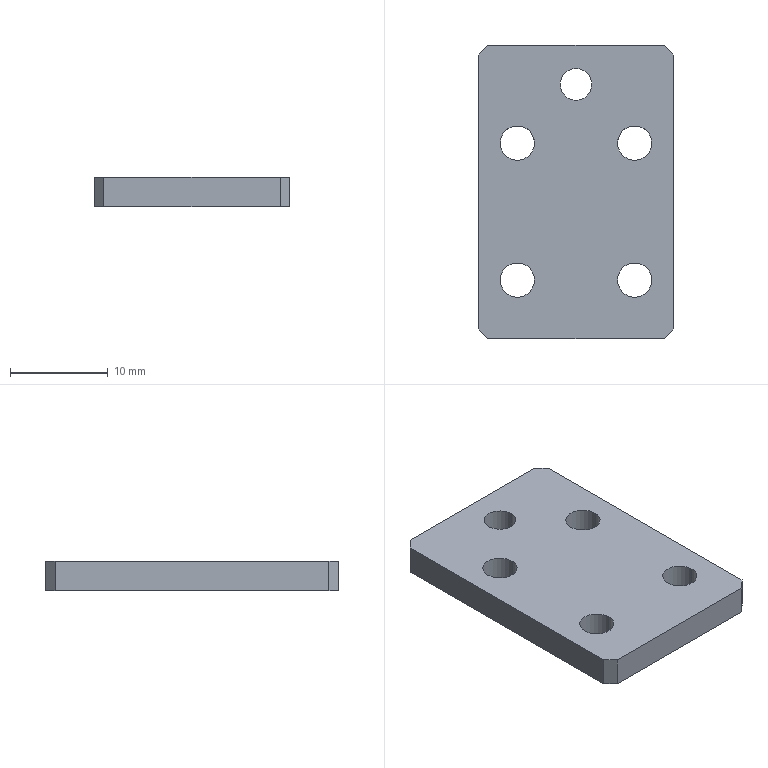Part | SolidWorks | features BaseBody 1 | 1 solid | 20 faces | box 20 x 30 x 3 mm | volume 1654 mm3 | cylinder 10 | plane 10 | commonest cylinder face diameters 3.5 x8 3.242 x2
STEP:
#1=CARTESIAN_POINT('',(30.706,86.212,0.));
#2=VERTEX_POINT('',#1);
#3=CARTESIAN_POINT('',(27.206,86.212,0.));
#4=VERTEX_POINT('',#3);
#5=CARTESIAN_POINT('',(28.956,86.212,0.));
#6=DIRECTION('',(0.,0.,-1.));
#7=DIRECTION('',(1.,0.,0.));
#8=AXIS2_PLACEMENT_3D('',#5,#6,#7);
#9=CIRCLE('',#8,1.75);
#10=EDGE_CURVE('',#2,#4,#9,.T.);
#11=ORIENTED_EDGE('',*,*,#10,.T.);
#12=CARTESIAN_POINT('',(27.206,86.212,3.));
#13=VERTEX_POINT('',#12);
#14=CARTESIAN_POINT('',(27.206,86.212,-33.18));
#15=DIRECTION('',(0.,0.,1.));
#16=VECTOR('',#15,1000.);
#17=LINE('',#14,#16);
#18=EDGE_CURVE('',#4,#13,#17,.T.);
#19=ORIENTED_EDGE('',*,*,#18,.T.);
#20=CARTESIAN_POINT('',(30.706,86.212,3.));
#21=VERTEX_POINT('',#20);
#22=CARTESIAN_POINT('',(28.956,86.212,3.));
#23=DIRECTION('',(0.,0.,-1.));
#24=DIRECTION('',(1.,0.,0.));
#25=AXIS2_PLACEMENT_3D('',#22,#23,#24);
#26=CIRCLE('',#25,1.75);
#27=EDGE_CURVE('',#21,#13,#26,.T.);
#28=ORIENTED_EDGE('',*,*,#27,.F.);
#29=CARTESIAN_POINT('',(30.706,86.212,-33.18));
#30=DIRECTION('',(0.,0.,1.));
#31=VECTOR('',#30,1000.);
#32=LINE('',#29,#31);
#33=EDGE_CURVE('',#2,#21,#32,.T.);
#34=ORIENTED_EDGE('',*,*,#33,.F.);
#35=EDGE_LOOP('',(#11,#19,#28,#34));
#36=FACE_OUTER_BOUND('',#35,.T.);
#37=CARTESIAN_POINT('',(28.956,86.212,-33.18));
#38=DIRECTION('',(0.,0.,1.));
#39=DIRECTION('',(1.,0.,0.));
#40=AXIS2_PLACEMENT_3D('',#37,#38,#39);
#41=CYLINDRICAL_SURFACE('',#40,1.75);
#42=ADVANCED_FACE('',(#36),#41,.F.);
#43=CARTESIAN_POINT('',(30.706,100.212,0.));
#44=VERTEX_POINT('',#43);
#45=CARTESIAN_POINT('',(27.206,100.212,0.));
#46=VERTEX_POINT('',#45);
#47=CARTESIAN_POINT('',(28.956,100.212,0.));
#48=DIRECTION('',(0.,0.,-1.));
#49=DIRECTION('',(1.,0.,0.));
#50=AXIS2_PLACEMENT_3D('',#47,#48,#49);
#51=CIRCLE('',#50,1.75);
#52=EDGE_CURVE('',#44,#46,#51,.T.);
#53=ORIENTED_EDGE('',*,*,#52,.T.);
#54=CARTESIAN_POINT('',(27.206,100.212,3.));
#55=VERTEX_POINT('',#54);
#56=CARTESIAN_POINT('',(27.206,100.212,-33.18));
#57=DIRECTION('',(0.,0.,1.));
#58=VECTOR('',#57,1000.);
#59=LINE('',#56,#58);
#60=EDGE_CURVE('',#46,#55,#59,.T.);
#61=ORIENTED_EDGE('',*,*,#60,.T.);
#62=CARTESIAN_POINT('',(30.706,100.212,3.));
#63=VERTEX_POINT('',#62);
#64=CARTESIAN_POINT('',(28.956,100.212,3.));
#65=DIRECTION('',(0.,0.,-1.));
#66=DIRECTION('',(1.,0.,0.));
#67=AXIS2_PLACEMENT_3D('',#64,#65,#66);
#68=CIRCLE('',#67,1.75);
#69=EDGE_CURVE('',#63,#55,#68,.T.);
#70=ORIENTED_EDGE('',*,*,#69,.F.);
#71=CARTESIAN_POINT('',(30.706,100.212,-33.18));
#72=DIRECTION('',(0.,0.,1.));
#73=VECTOR('',#72,1000.);
#74=LINE('',#71,#73);
#75=EDGE_CURVE('',#44,#63,#74,.T.);
#76=ORIENTED_EDGE('',*,*,#75,.F.);
#77=EDGE_LOOP('',(#53,#61,#70,#76));
#78=FACE_OUTER_BOUND('',#77,.T.);
#79=CARTESIAN_POINT('',(28.956,100.212,-33.18));
#80=DIRECTION('',(0.,0.,1.));
#81=DIRECTION('',(1.,0.,0.));
#82=AXIS2_PLACEMENT_3D('',#79,#80,#81);
#83=CYLINDRICAL_SURFACE('',#82,1.75);
#84=ADVANCED_FACE('',(#78),#83,.F.);
#85=CARTESIAN_POINT('',(18.706,100.212,0.));
#86=VERTEX_POINT('',#85);
#87=CARTESIAN_POINT('',(15.206,100.212,0.));
#88=VERTEX_POINT('',#87);
#89=CARTESIAN_POINT('',(16.956,100.212,0.));
#90=DIRECTION('',(0.,0.,-1.));
#91=DIRECTION('',(1.,0.,0.));
#92=AXIS2_PLACEMENT_3D('',#89,#90,#91);
#93=CIRCLE('',#92,1.75);
#94=EDGE_CURVE('',#86,#88,#93,.T.);
#95=ORIENTED_EDGE('',*,*,#94,.T.);
#96=CARTESIAN_POINT('',(15.206,100.212,3.));
#97=VERTEX_POINT('',#96);
#98=CARTESIAN_POINT('',(15.206,100.212,-33.18));
#99=DIRECTION('',(0.,0.,1.));
#100=VECTOR('',#99,1000.);
#101=LINE('',#98,#100);
#102=EDGE_CURVE('',#88,#97,#101,.T.);
#103=ORIENTED_EDGE('',*,*,#102,.T.);
#104=CARTESIAN_POINT('',(18.706,100.212,3.));
#105=VERTEX_POINT('',#104);
#106=CARTESIAN_POINT('',(16.956,100.212,3.));
#107=DIRECTION('',(0.,0.,-1.));
#108=DIRECTION('',(1.,0.,0.));
#109=AXIS2_PLACEMENT_3D('',#106,#107,#108);
#110=CIRCLE('',#109,1.75);
#111=EDGE_CURVE('',#105,#97,#110,.T.);
#112=ORIENTED_EDGE('',*,*,#111,.F.);
#113=CARTESIAN_POINT('',(18.706,100.212,-33.18));
#114=DIRECTION('',(0.,0.,1.));
#115=VECTOR('',#114,1000.);
#116=LINE('',#113,#115);
#117=EDGE_CURVE('',#86,#105,#116,.T.);
#118=ORIENTED_EDGE('',*,*,#117,.F.);
#119=EDGE_LOOP('',(#95,#103,#112,#118));
#120=FACE_OUTER_BOUND('',#119,.T.);
#121=CARTESIAN_POINT('',(16.956,100.212,-33.18));
#122=DIRECTION('',(0.,0.,1.));
#123=DIRECTION('',(1.,0.,0.));
#124=AXIS2_PLACEMENT_3D('',#121,#122,#123);
#125=CYLINDRICAL_SURFACE('',#124,1.75);
#126=ADVANCED_FACE('',(#120),#125,.F.);
#127=CARTESIAN_POINT('',(18.706,86.212,0.));
#128=VERTEX_POINT('',#127);
#129=CARTESIAN_POINT('',(15.206,86.212,0.));
#130=VERTEX_POINT('',#129);
#131=CARTESIAN_POINT('',(16.956,86.212,0.));
#132=DIRECTION('',(0.,0.,-1.));
#133=DIRECTION('',(1.,0.,0.));
#134=AXIS2_PLACEMENT_3D('',#131,#132,#133);
#135=CIRCLE('',#134,1.75);
#136=EDGE_CURVE('',#128,#130,#135,.T.);
#137=ORIENTED_EDGE('',*,*,#136,.T.);
#138=CARTESIAN_POINT('',(15.206,86.212,3.));
#139=VERTEX_POINT('',#138);
#140=CARTESIAN_POINT('',(15.206,86.212,-33.18));
#141=DIRECTION('',(0.,0.,1.));
#142=VECTOR('',#141,1000.);
#143=LINE('',#140,#142);
#144=EDGE_CURVE('',#130,#139,#143,.T.);
#145=ORIENTED_EDGE('',*,*,#144,.T.);
#146=CARTESIAN_POINT('',(18.706,86.212,3.));
#147=VERTEX_POINT('',#146);
#148=CARTESIAN_POINT('',(16.956,86.212,3.));
#149=DIRECTION('',(0.,0.,-1.));
#150=DIRECTION('',(1.,0.,0.));
#151=AXIS2_PLACEMENT_3D('',#148,#149,#150);
#152=CIRCLE('',#151,1.75);
#153=EDGE_CURVE('',#147,#139,#152,.T.);
#154=ORIENTED_EDGE('',*,*,#153,.F.);
#155=CARTESIAN_POINT('',(18.706,86.212,-33.18));
#156=DIRECTION('',(0.,0.,1.));
#157=VECTOR('',#156,1000.);
#158=LINE('',#155,#157);
#159=EDGE_CURVE('',#128,#147,#158,.T.);
#160=ORIENTED_EDGE('',*,*,#159,.F.);
#161=EDGE_LOOP('',(#137,#145,#154,#160));
#162=FACE_OUTER_BOUND('',#161,.T.);
#163=CARTESIAN_POINT('',(16.956,86.212,-33.18));
#164=DIRECTION('',(0.,0.,1.));
#165=DIRECTION('',(1.,0.,0.));
#166=AXIS2_PLACEMENT_3D('',#163,#164,#165);
#167=CYLINDRICAL_SURFACE('',#166,1.75);
#168=ADVANCED_FACE('',(#162),#167,.F.);
#169=CARTESIAN_POINT('',(24.577,106.212,0.));
#170=VERTEX_POINT('',#169);
#171=CARTESIAN_POINT('',(21.335,106.212,0.));
#172=VERTEX_POINT('',#171);
#173=CARTESIAN_POINT('',(22.956,106.212,0.));
#174=DIRECTION('',(0.,0.,-1.));
#175=DIRECTION('',(1.,0.,0.));
#176=AXIS2_PLACEMENT_3D('',#173,#174,#175);
#177=CIRCLE('',#176,1.621);
#178=EDGE_CURVE('',#170,#172,#177,.T.);
#179=ORIENTED_EDGE('',*,*,#178,.T.);
#180=CARTESIAN_POINT('',(21.335,106.212,3.));
#181=VERTEX_POINT('',#180);
#182=CARTESIAN_POINT('',(21.335,106.212,-33.18));
#183=DIRECTION('',(0.,0.,1.));
#184=VECTOR('',#183,1000.);
#185=LINE('',#182,#184);
#186=EDGE_CURVE('',#172,#181,#185,.T.);
#187=ORIENTED_EDGE('',*,*,#186,.T.);
#188=CARTESIAN_POINT('',(24.577,106.212,3.));
#189=VERTEX_POINT('',#188);
#190=CARTESIAN_POINT('',(22.956,106.212,3.));
#191=DIRECTION('',(0.,0.,-1.));
#192=DIRECTION('',(1.,0.,0.));
#193=AXIS2_PLACEMENT_3D('',#190,#191,#192);
#194=CIRCLE('',#193,1.621);
#195=EDGE_CURVE('',#189,#181,#194,.T.);
#196=ORIENTED_EDGE('',*,*,#195,.F.);
#197=CARTESIAN_POINT('',(24.577,106.212,-33.18));
#198=DIRECTION('',(0.,0.,1.));
#199=VECTOR('',#198,1000.);
#200=LINE('',#197,#199);
#201=EDGE_CURVE('',#170,#189,#200,.T.);
#202=ORIENTED_EDGE('',*,*,#201,.F.);
#203=EDGE_LOOP('',(#179,#187,#196,#202));
#204=FACE_OUTER_BOUND('',#203,.T.);
#205=CARTESIAN_POINT('',(22.956,106.212,-33.18));
#206=DIRECTION('',(0.,0.,1.));
#207=DIRECTION('',(1.,0.,0.));
#208=AXIS2_PLACEMENT_3D('',#205,#206,#207);
#209=CYLINDRICAL_SURFACE('',#208,1.621);
#210=ADVANCED_FACE('',(#204),#209,.F.);
#211=ORIENTED_EDGE('',*,*,#10,.F.);
#212=CARTESIAN_POINT('',(28.956,86.212,0.));
#213=DIRECTION('',(0.,0.,-1.));
#214=DIRECTION('',(1.,0.,0.));
#215=AXIS2_PLACEMENT_3D('',#212,#213,#214);
#216=CIRCLE('',#215,1.75);
#217=EDGE_CURVE('',#4,#2,#216,.T.);
#218=ORIENTED_EDGE('',*,*,#217,.F.);
#219=EDGE_LOOP('',(#211,#218));
#220=FACE_BOUND('',#219,.T.);
#221=ORIENTED_EDGE('',*,*,#52,.F.);
#222=CARTESIAN_POINT('',(28.956,100.212,0.));
#223=DIRECTION('',(0.,0.,-1.));
#224=DIRECTION('',(1.,0.,0.));
#225=AXIS2_PLACEMENT_3D('',#222,#223,#224);
#226=CIRCLE('',#225,1.75);
#227=EDGE_CURVE('',#46,#44,#226,.T.);
#228=ORIENTED_EDGE('',*,*,#227,.F.);
#229=EDGE_LOOP('',(#221,#228));
#230=FACE_BOUND('',#229,.T.);
#231=ORIENTED_EDGE('',*,*,#94,.F.);
#232=CARTESIAN_POINT('',(16.956,100.212,0.));
#233=DIRECTION('',(0.,0.,-1.));
#234=DIRECTION('',(1.,0.,0.));
#235=AXIS2_PLACEMENT_3D('',#232,#233,#234);
#236=CIRCLE('',#235,1.75);
#237=EDGE_CURVE('',#88,#86,#236,.T.);
#238=ORIENTED_EDGE('',*,*,#237,.F.);
#239=EDGE_LOOP('',(#231,#238));
#240=FACE_BOUND('',#239,.T.);
#241=ORIENTED_EDGE('',*,*,#136,.F.);
#242=CARTESIAN_POINT('',(16.956,86.212,0.));
#243=DIRECTION('',(0.,0.,-1.));
#244=DIRECTION('',(1.,0.,0.));
#245=AXIS2_PLACEMENT_3D('',#242,#243,#244);
#246=CIRCLE('',#245,1.75);
#247=EDGE_CURVE('',#130,#128,#246,.T.);
#248=ORIENTED_EDGE('',*,*,#247,.F.);
#249=EDGE_LOOP('',(#241,#248));
#250=FACE_BOUND('',#249,.T.);
#251=ORIENTED_EDGE('',*,*,#178,.F.);
#252=CARTESIAN_POINT('',(22.956,106.212,0.));
#253=DIRECTION('',(0.,0.,-1.));
#254=DIRECTION('',(1.,0.,0.));
#255=AXIS2_PLACEMENT_3D('',#252,#253,#254);
#256=CIRCLE('',#255,1.621);
#257=EDGE_CURVE('',#172,#170,#256,.T.);
#258=ORIENTED_EDGE('',*,*,#257,.F.);
#259=EDGE_LOOP('',(#251,#258));
#260=FACE_BOUND('',#259,.T.);
#261=CARTESIAN_POINT('',(32.956,81.212,0.));
#262=VERTEX_POINT('',#261);
#263=CARTESIAN_POINT('',(32.956,109.212,0.));
#264=VERTEX_POINT('',#263);
#265=CARTESIAN_POINT('',(32.956,95.212,0.));
#266=DIRECTION('',(0.,1.,0.));
#267=VECTOR('',#266,1000.);
#268=LINE('',#265,#267);
#269=EDGE_CURVE('',#262,#264,#268,.T.);
#270=ORIENTED_EDGE('',*,*,#269,.F.);
#271=CARTESIAN_POINT('',(31.956,80.212,0.));
#272=VERTEX_POINT('',#271);
#273=CARTESIAN_POINT('',(32.456,80.712,0.));
#274=DIRECTION('',(0.7071,0.7071,0.));
#275=VECTOR('',#274,1000.);
#276=LINE('',#273,#275);
#277=EDGE_CURVE('',#272,#262,#276,.T.);
#278=ORIENTED_EDGE('',*,*,#277,.F.);
#279=CARTESIAN_POINT('',(13.956,80.212,0.));
#280=VERTEX_POINT('',#279);
#281=CARTESIAN_POINT('',(22.956,80.212,0.));
#282=DIRECTION('',(1.,0.,0.));
#283=VECTOR('',#282,1000.);
#284=LINE('',#281,#283);
#285=EDGE_CURVE('',#280,#272,#284,.T.);
#286=ORIENTED_EDGE('',*,*,#285,.F.);
#287=CARTESIAN_POINT('',(12.956,81.212,0.));
#288=VERTEX_POINT('',#287);
#289=CARTESIAN_POINT('',(13.456,80.712,0.));
#290=DIRECTION('',(0.7071,-0.7071,0.));
#291=VECTOR('',#290,1000.);
#292=LINE('',#289,#291);
#293=EDGE_CURVE('',#288,#280,#292,.T.);
#294=ORIENTED_EDGE('',*,*,#293,.F.);
#295=CARTESIAN_POINT('',(12.956,109.212,0.));
#296=VERTEX_POINT('',#295);
#297=CARTESIAN_POINT('',(12.956,95.212,0.));
#298=DIRECTION('',(0.,-1.,0.));
#299=VECTOR('',#298,1000.);
#300=LINE('',#297,#299);
#301=EDGE_CURVE('',#296,#288,#300,.T.);
#302=ORIENTED_EDGE('',*,*,#301,.F.);
#303=CARTESIAN_POINT('',(13.956,110.212,0.));
#304=VERTEX_POINT('',#303);
#305=CARTESIAN_POINT('',(13.456,109.712,0.));
#306=DIRECTION('',(-0.7071,-0.7071,0.));
#307=VECTOR('',#306,1000.);
#308=LINE('',#305,#307);
#309=EDGE_CURVE('',#304,#296,#308,.T.);
#310=ORIENTED_EDGE('',*,*,#309,.F.);
#311=CARTESIAN_POINT('',(31.956,110.212,0.));
#312=VERTEX_POINT('',#311);
#313=CARTESIAN_POINT('',(22.956,110.212,0.));
#314=DIRECTION('',(-1.,0.,0.));
#315=VECTOR('',#314,1000.);
#316=LINE('',#313,#315);
#317=EDGE_CURVE('',#312,#304,#316,.T.);
#318=ORIENTED_EDGE('',*,*,#317,.F.);
#319=CARTESIAN_POINT('',(32.456,109.712,0.));
#320=DIRECTION('',(-0.7071,0.7071,0.));
#321=VECTOR('',#320,1000.);
#322=LINE('',#319,#321);
#323=EDGE_CURVE('',#264,#312,#322,.T.);
#324=ORIENTED_EDGE('',*,*,#323,.F.);
#325=EDGE_LOOP('',(#270,#278,#286,#294,#302,#310,#318,#324));
#326=FACE_OUTER_BOUND('',#325,.T.);
#327=CARTESIAN_POINT('',(22.956,95.212,0.));
#328=DIRECTION('',(0.,0.,1.));
#329=DIRECTION('',(1.,0.,0.));
#330=AXIS2_PLACEMENT_3D('',#327,#328,#329);
#331=PLANE('',#330);
#332=ADVANCED_FACE('',(#220,#230,#240,#250,#260,#326),#331,.F.);
#333=ORIENTED_EDGE('',*,*,#18,.F.);
#334=ORIENTED_EDGE('',*,*,#217,.T.);
#335=ORIENTED_EDGE('',*,*,#33,.T.);
#336=CARTESIAN_POINT('',(28.956,86.212,3.));
#337=DIRECTION('',(0.,0.,-1.));
#338=DIRECTION('',(1.,0.,0.));
#339=AXIS2_PLACEMENT_3D('',#336,#337,#338);
#340=CIRCLE('',#339,1.75);
#341=EDGE_CURVE('',#13,#21,#340,.T.);
#342=ORIENTED_EDGE('',*,*,#341,.F.);
#343=EDGE_LOOP('',(#333,#334,#335,#342));
#344=FACE_OUTER_BOUND('',#343,.T.);
#345=CARTESIAN_POINT('',(28.956,86.212,-33.18));
#346=DIRECTION('',(0.,0.,1.));
#347=DIRECTION('',(1.,0.,0.));
#348=AXIS2_PLACEMENT_3D('',#345,#346,#347);
#349=CYLINDRICAL_SURFACE('',#348,1.75);
#350=ADVANCED_FACE('',(#344),#349,.F.);
#351=ORIENTED_EDGE('',*,*,#60,.F.);
#352=ORIENTED_EDGE('',*,*,#227,.T.);
#353=ORIENTED_EDGE('',*,*,#75,.T.);
#354=CARTESIAN_POINT('',(28.956,100.212,3.));
#355=DIRECTION('',(0.,0.,-1.));
#356=DIRECTION('',(1.,0.,0.));
#357=AXIS2_PLACEMENT_3D('',#354,#355,#356);
#358=CIRCLE('',#357,1.75);
#359=EDGE_CURVE('',#55,#63,#358,.T.);
#360=ORIENTED_EDGE('',*,*,#359,.F.);
#361=EDGE_LOOP('',(#351,#352,#353,#360));
#362=FACE_OUTER_BOUND('',#361,.T.);
#363=CARTESIAN_POINT('',(28.956,100.212,-33.18));
#364=DIRECTION('',(0.,0.,1.));
#365=DIRECTION('',(1.,0.,0.));
#366=AXIS2_PLACEMENT_3D('',#363,#364,#365);
#367=CYLINDRICAL_SURFACE('',#366,1.75);
#368=ADVANCED_FACE('',(#362),#367,.F.);
#369=ORIENTED_EDGE('',*,*,#102,.F.);
#370=ORIENTED_EDGE('',*,*,#237,.T.);
#371=ORIENTED_EDGE('',*,*,#117,.T.);
#372=CARTESIAN_POINT('',(16.956,100.212,3.));
#373=DIRECTION('',(0.,0.,-1.));
#374=DIRECTION('',(1.,0.,0.));
#375=AXIS2_PLACEMENT_3D('',#372,#373,#374);
#376=CIRCLE('',#375,1.75);
#377=EDGE_CURVE('',#97,#105,#376,.T.);
#378=ORIENTED_EDGE('',*,*,#377,.F.);
#379=EDGE_LOOP('',(#369,#370,#371,#378));
#380=FACE_OUTER_BOUND('',#379,.T.);
#381=CARTESIAN_POINT('',(16.956,100.212,-33.18));
#382=DIRECTION('',(0.,0.,1.));
#383=DIRECTION('',(1.,0.,0.));
#384=AXIS2_PLACEMENT_3D('',#381,#382,#383);
#385=CYLINDRICAL_SURFACE('',#384,1.75);
#386=ADVANCED_FACE('',(#380),#385,.F.);
#387=ORIENTED_EDGE('',*,*,#144,.F.);
#388=ORIENTED_EDGE('',*,*,#247,.T.);
#389=ORIENTED_EDGE('',*,*,#159,.T.);
#390=CARTESIAN_POINT('',(16.956,86.212,3.));
#391=DIRECTION('',(0.,0.,-1.));
#392=DIRECTION('',(1.,0.,0.));
#393=AXIS2_PLACEMENT_3D('',#390,#391,#392);
#394=CIRCLE('',#393,1.75);
#395=EDGE_CURVE('',#139,#147,#394,.T.);
#396=ORIENTED_EDGE('',*,*,#395,.F.);
#397=EDGE_LOOP('',(#387,#388,#389,#396));
#398=FACE_OUTER_BOUND('',#397,.T.);
#399=CARTESIAN_POINT('',(16.956,86.212,-33.18));
#400=DIRECTION('',(0.,0.,1.));
#401=DIRECTION('',(1.,0.,0.));
#402=AXIS2_PLACEMENT_3D('',#399,#400,#401);
#403=CYLINDRICAL_SURFACE('',#402,1.75);
#404=ADVANCED_FACE('',(#398),#403,.F.);
#405=ORIENTED_EDGE('',*,*,#186,.F.);
#406=ORIENTED_EDGE('',*,*,#257,.T.);
#407=ORIENTED_EDGE('',*,*,#201,.T.);
#408=CARTESIAN_POINT('',(22.956,106.212,3.));
#409=DIRECTION('',(0.,0.,-1.));
#410=DIRECTION('',(1.,0.,0.));
#411=AXIS2_PLACEMENT_3D('',#408,#409,#410);
#412=CIRCLE('',#411,1.621);
#413=EDGE_CURVE('',#181,#189,#412,.T.);
#414=ORIENTED_EDGE('',*,*,#413,.F.);
#415=EDGE_LOOP('',(#405,#406,#407,#414));
#416=FACE_OUTER_BOUND('',#415,.T.);
#417=CARTESIAN_POINT('',(22.956,106.212,-33.18));
#418=DIRECTION('',(0.,0.,1.));
#419=DIRECTION('',(1.,0.,0.));
#420=AXIS2_PLACEMENT_3D('',#417,#418,#419);
#421=CYLINDRICAL_SURFACE('',#420,1.621);
#422=ADVANCED_FACE('',(#416),#421,.F.);
#423=CARTESIAN_POINT('',(32.956,81.212,3.));
#424=VERTEX_POINT('',#423);
#425=CARTESIAN_POINT('',(32.956,81.212,0.));
#426=DIRECTION('',(0.,0.,-1.));
#427=VECTOR('',#426,1000.);
#428=LINE('',#425,#427);
#429=EDGE_CURVE('',#424,#262,#428,.T.);
#430=ORIENTED_EDGE('',*,*,#429,.T.);
#431=ORIENTED_EDGE('',*,*,#269,.T.);
#432=CARTESIAN_POINT('',(32.956,109.212,3.));
#433=VERTEX_POINT('',#432);
#434=CARTESIAN_POINT('',(32.956,109.212,0.));
#435=DIRECTION('',(0.,0.,1.));
#436=VECTOR('',#435,1000.);
#437=LINE('',#434,#436);
#438=EDGE_CURVE('',#264,#433,#437,.T.);
#439=ORIENTED_EDGE('',*,*,#438,.T.);
#440=CARTESIAN_POINT('',(32.956,110.212,3.));
#441=DIRECTION('',(0.,-1.,0.));
#442=VECTOR('',#441,1000.);
#443=LINE('',#440,#442);
#444=EDGE_CURVE('',#433,#424,#443,.T.);
#445=ORIENTED_EDGE('',*,*,#444,.T.);
#446=EDGE_LOOP('',(#430,#431,#439,#445));
#447=FACE_OUTER_BOUND('',#446,.T.);
#448=CARTESIAN_POINT('',(32.956,110.212,0.));
#449=DIRECTION('',(1.,0.,0.));
#450=DIRECTION('',(0.,0.,-1.));
#451=AXIS2_PLACEMENT_3D('',#448,#449,#450);
#452=PLANE('',#451);
#453=ADVANCED_FACE('',(#447),#452,.T.);
#454=CARTESIAN_POINT('',(13.956,80.212,3.));
#455=VERTEX_POINT('',#454);
#456=CARTESIAN_POINT('',(13.956,80.212,0.));
#457=DIRECTION('',(0.,0.,-1.));
#458=VECTOR('',#457,1000.);
#459=LINE('',#456,#458);
#460=EDGE_CURVE('',#455,#280,#459,.T.);
#461=ORIENTED_EDGE('',*,*,#460,.T.);
#462=ORIENTED_EDGE('',*,*,#285,.T.);
#463=CARTESIAN_POINT('',(31.956,80.212,3.));
#464=VERTEX_POINT('',#463);
#465=CARTESIAN_POINT('',(31.956,80.212,0.));
#466=DIRECTION('',(0.,0.,1.));
#467=VECTOR('',#466,1000.);
#468=LINE('',#465,#467);
#469=EDGE_CURVE('',#272,#464,#468,.T.);
#470=ORIENTED_EDGE('',*,*,#469,.T.);
#471=CARTESIAN_POINT('',(32.956,80.212,3.));
#472=DIRECTION('',(-1.,0.,0.));
#473=VECTOR('',#472,1000.);
#474=LINE('',#471,#473);
#475=EDGE_CURVE('',#464,#455,#474,.T.);
#476=ORIENTED_EDGE('',*,*,#475,.T.);
#477=EDGE_LOOP('',(#461,#462,#470,#476));
#478=FACE_OUTER_BOUND('',#477,.T.);
#479=CARTESIAN_POINT('',(32.956,80.212,0.));
#480=DIRECTION('',(0.,-1.,0.));
#481=DIRECTION('',(0.,0.,-1.));
#482=AXIS2_PLACEMENT_3D('',#479,#480,#481);
#483=PLANE('',#482);
#484=ADVANCED_FACE('',(#478),#483,.T.);
#485=CARTESIAN_POINT('',(12.956,109.212,3.));
#486=VERTEX_POINT('',#485);
#487=CARTESIAN_POINT('',(12.956,109.212,0.));
#488=DIRECTION('',(0.,0.,-1.));
#489=VECTOR('',#488,1000.);
#490=LINE('',#487,#489);
#491=EDGE_CURVE('',#486,#296,#490,.T.);
#492=ORIENTED_EDGE('',*,*,#491,.T.);
#493=ORIENTED_EDGE('',*,*,#301,.T.);
#494=CARTESIAN_POINT('',(12.956,81.212,3.));
#495=VERTEX_POINT('',#494);
#496=CARTESIAN_POINT('',(12.956,81.212,0.));
#497=DIRECTION('',(0.,0.,1.));
#498=VECTOR('',#497,1000.);
#499=LINE('',#496,#498);
#500=EDGE_CURVE('',#288,#495,#499,.T.);
#501=ORIENTED_EDGE('',*,*,#500,.T.);
#502=CARTESIAN_POINT('',(12.956,80.212,3.));
#503=DIRECTION('',(0.,1.,0.));
#504=VECTOR('',#503,1000.);
#505=LINE('',#502,#504);
#506=EDGE_CURVE('',#495,#486,#505,.T.);
#507=ORIENTED_EDGE('',*,*,#506,.T.);
#508=EDGE_LOOP('',(#492,#493,#501,#507));
#509=FACE_OUTER_BOUND('',#508,.T.);
#510=CARTESIAN_POINT('',(12.956,80.212,0.));
#511=DIRECTION('',(-1.,0.,0.));
#512=DIRECTION('',(0.,0.,1.));
#513=AXIS2_PLACEMENT_3D('',#510,#511,#512);
#514=PLANE('',#513);
#515=ADVANCED_FACE('',(#509),#514,.T.);
#516=CARTESIAN_POINT('',(13.956,110.212,3.));
#517=VERTEX_POINT('',#516);
#518=CARTESIAN_POINT('',(13.956,110.212,0.));
#519=DIRECTION('',(0.,0.,1.));
#520=VECTOR('',#519,1000.);
#521=LINE('',#518,#520);
#522=EDGE_CURVE('',#304,#517,#521,.T.);
#523=ORIENTED_EDGE('',*,*,#522,.T.);
#524=CARTESIAN_POINT('',(31.956,110.212,3.));
#525=VERTEX_POINT('',#524);
#526=CARTESIAN_POINT('',(12.956,110.212,3.));
#527=DIRECTION('',(1.,0.,0.));
#528=VECTOR('',#527,1000.);
#529=LINE('',#526,#528);
#530=EDGE_CURVE('',#517,#525,#529,.T.);
#531=ORIENTED_EDGE('',*,*,#530,.T.);
#532=CARTESIAN_POINT('',(31.956,110.212,0.));
#533=DIRECTION('',(0.,0.,-1.));
#534=VECTOR('',#533,1000.);
#535=LINE('',#532,#534);
#536=EDGE_CURVE('',#525,#312,#535,.T.);
#537=ORIENTED_EDGE('',*,*,#536,.T.);
#538=ORIENTED_EDGE('',*,*,#317,.T.);
#539=EDGE_LOOP('',(#523,#531,#537,#538));
#540=FACE_OUTER_BOUND('',#539,.T.);
#541=CARTESIAN_POINT('',(12.956,110.212,0.));
#542=DIRECTION('',(0.,1.,0.));
#543=DIRECTION('',(0.,0.,1.));
#544=AXIS2_PLACEMENT_3D('',#541,#542,#543);
#545=PLANE('',#544);
#546=ADVANCED_FACE('',(#540),#545,.T.);
#547=ORIENTED_EDGE('',*,*,#27,.T.);
#548=ORIENTED_EDGE('',*,*,#341,.T.);
#549=EDGE_LOOP('',(#547,#548));
#550=FACE_BOUND('',#549,.T.);
#551=ORIENTED_EDGE('',*,*,#69,.T.);
#552=ORIENTED_EDGE('',*,*,#359,.T.);
#553=EDGE_LOOP('',(#551,#552));
#554=FACE_BOUND('',#553,.T.);
#555=ORIENTED_EDGE('',*,*,#111,.T.);
#556=ORIENTED_EDGE('',*,*,#377,.T.);
#557=EDGE_LOOP('',(#555,#556));
#558=FACE_BOUND('',#557,.T.);
#559=ORIENTED_EDGE('',*,*,#153,.T.);
#560=ORIENTED_EDGE('',*,*,#395,.T.);
#561=EDGE_LOOP('',(#559,#560));
#562=FACE_BOUND('',#561,.T.);
#563=ORIENTED_EDGE('',*,*,#195,.T.);
#564=ORIENTED_EDGE('',*,*,#413,.T.);
#565=EDGE_LOOP('',(#563,#564));
#566=FACE_BOUND('',#565,.T.);
#567=CARTESIAN_POINT('',(31.956,80.212,3.));
#568=DIRECTION('',(0.7071,0.7071,0.));
#569=VECTOR('',#568,1000.);
#570=LINE('',#567,#569);
#571=EDGE_CURVE('',#464,#424,#570,.T.);
#572=ORIENTED_EDGE('',*,*,#571,.T.);
#573=ORIENTED_EDGE('',*,*,#444,.F.);
#574=CARTESIAN_POINT('',(32.956,109.212,3.));
#575=DIRECTION('',(-0.7071,0.7071,0.));
#576=VECTOR('',#575,1000.);
#577=LINE('',#574,#576);
#578=EDGE_CURVE('',#433,#525,#577,.T.);
#579=ORIENTED_EDGE('',*,*,#578,.T.);
#580=ORIENTED_EDGE('',*,*,#530,.F.);
#581=CARTESIAN_POINT('',(13.956,110.212,3.));
#582=DIRECTION('',(-0.7071,-0.7071,0.));
#583=VECTOR('',#582,1000.);
#584=LINE('',#581,#583);
#585=EDGE_CURVE('',#517,#486,#584,.T.);
#586=ORIENTED_EDGE('',*,*,#585,.T.);
#587=ORIENTED_EDGE('',*,*,#506,.F.);
#588=CARTESIAN_POINT('',(12.956,81.212,3.));
#589=DIRECTION('',(0.7071,-0.7071,0.));
#590=VECTOR('',#589,1000.);
#591=LINE('',#588,#590);
#592=EDGE_CURVE('',#495,#455,#591,.T.);
#593=ORIENTED_EDGE('',*,*,#592,.T.);
#594=ORIENTED_EDGE('',*,*,#475,.F.);
#595=EDGE_LOOP('',(#572,#573,#579,#580,#586,#587,#593,#594));
#596=FACE_OUTER_BOUND('',#595,.T.);
#597=CARTESIAN_POINT('',(22.956,95.212,3.));
#598=DIRECTION('',(0.,0.,1.));
#599=DIRECTION('',(1.,0.,0.));
#600=AXIS2_PLACEMENT_3D('',#597,#598,#599);
#601=PLANE('',#600);
#602=ADVANCED_FACE('',(#550,#554,#558,#562,#566,#596),#601,.T.);
#603=ORIENTED_EDGE('',*,*,#277,.T.);
#604=ORIENTED_EDGE('',*,*,#429,.F.);
#605=ORIENTED_EDGE('',*,*,#571,.F.);
#606=ORIENTED_EDGE('',*,*,#469,.F.);
#607=EDGE_LOOP('',(#603,#604,#605,#606));
#608=FACE_OUTER_BOUND('',#607,.T.);
#609=CARTESIAN_POINT('',(32.456,80.712,0.));
#610=DIRECTION('',(0.7071,-0.7071,0.));
#611=DIRECTION('',(0.7071,0.7071,0.));
#612=AXIS2_PLACEMENT_3D('',#609,#610,#611);
#613=PLANE('',#612);
#614=ADVANCED_FACE('',(#608),#613,.T.);
#615=ORIENTED_EDGE('',*,*,#323,.T.);
#616=ORIENTED_EDGE('',*,*,#536,.F.);
#617=ORIENTED_EDGE('',*,*,#578,.F.);
#618=ORIENTED_EDGE('',*,*,#438,.F.);
#619=EDGE_LOOP('',(#615,#616,#617,#618));
#620=FACE_OUTER_BOUND('',#619,.T.);
#621=CARTESIAN_POINT('',(32.456,109.712,0.));
#622=DIRECTION('',(0.7071,0.7071,0.));
#623=DIRECTION('',(-0.7071,0.7071,0.));
#624=AXIS2_PLACEMENT_3D('',#621,#622,#623);
#625=PLANE('',#624);
#626=ADVANCED_FACE('',(#620),#625,.T.);
#627=ORIENTED_EDGE('',*,*,#293,.T.);
#628=ORIENTED_EDGE('',*,*,#460,.F.);
#629=ORIENTED_EDGE('',*,*,#592,.F.);
#630=ORIENTED_EDGE('',*,*,#500,.F.);
#631=EDGE_LOOP('',(#627,#628,#629,#630));
#632=FACE_OUTER_BOUND('',#631,.T.);
#633=CARTESIAN_POINT('',(13.456,80.712,0.));
#634=DIRECTION('',(-0.7071,-0.7071,0.));
#635=DIRECTION('',(0.7071,-0.7071,0.));
#636=AXIS2_PLACEMENT_3D('',#633,#634,#635);
#637=PLANE('',#636);
#638=ADVANCED_FACE('',(#632),#637,.T.);
#639=ORIENTED_EDGE('',*,*,#309,.T.);
#640=ORIENTED_EDGE('',*,*,#491,.F.);
#641=ORIENTED_EDGE('',*,*,#585,.F.);
#642=ORIENTED_EDGE('',*,*,#522,.F.);
#643=EDGE_LOOP('',(#639,#640,#641,#642));
#644=FACE_OUTER_BOUND('',#643,.T.);
#645=CARTESIAN_POINT('',(13.456,109.712,0.));
#646=DIRECTION('',(-0.7071,0.7071,0.));
#647=DIRECTION('',(-0.7071,-0.7071,0.));
#648=AXIS2_PLACEMENT_3D('',#645,#646,#647);
#649=PLANE('',#648);
#650=ADVANCED_FACE('',(#644),#649,.T.);
#651=CLOSED_SHELL('',(#42,#84,#126,#168,#210,#332,#350,#368,#386,#404,#422,#453,#484,#515,#546,#602,#614,#626,#638,#650));
#652=MANIFOLD_SOLID_BREP('',#651);
#653=CARTESIAN_POINT('',(0.,0.,0.));
#654=DIRECTION('',(0.,0.,1.));
#655=DIRECTION('',(1.,0.,0.));
#656=AXIS2_PLACEMENT_3D('',#653,#654,#655);
#657=(LENGTH_UNIT()NAMED_UNIT(*)SI_UNIT(.MILLI.,.METRE.));
#658=UNCERTAINTY_MEASURE_WITH_UNIT(LENGTH_MEASURE(0.00001),#657,'','');
#659=(NAMED_UNIT(*)PLANE_ANGLE_UNIT()SI_UNIT($,.RADIAN.));
#660=(NAMED_UNIT(*)SI_UNIT($,.STERADIAN.)SOLID_ANGLE_UNIT());
#661=(GEOMETRIC_REPRESENTATION_CONTEXT(3)GLOBAL_UNCERTAINTY_ASSIGNED_CONTEXT((#658))GLOBAL_UNIT_ASSIGNED_CONTEXT((#657,#659,#660))REPRESENTATION_CONTEXT('',''));
#662=ADVANCED_BREP_SHAPE_REPRESENTATION('',(#652,#656),#661);